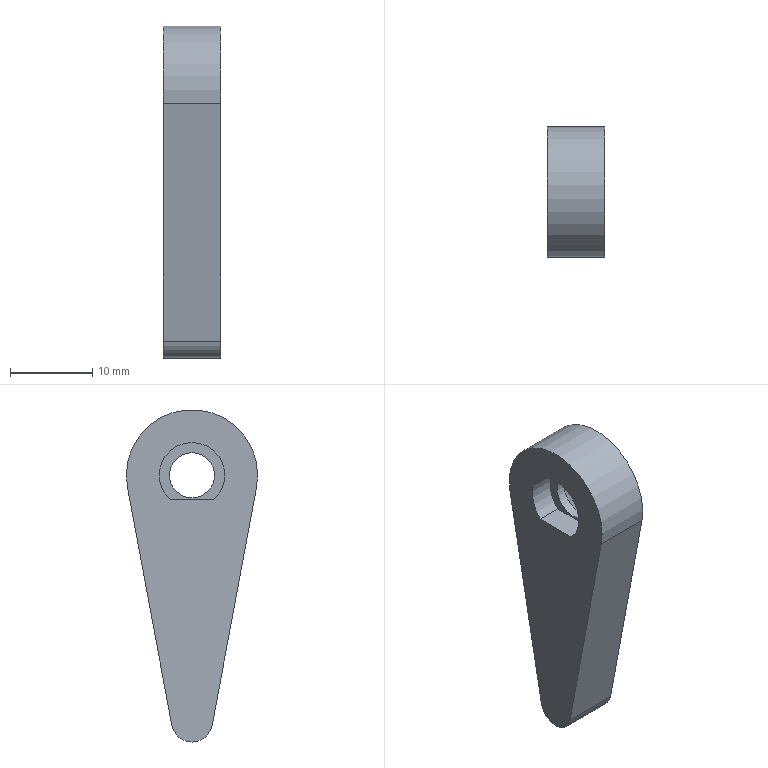Part | NX | features DATUM_CSYS 2, EXTRUDE 2, SKETCH 2, CSUNK_HOLE 1, HOLE PACKAGE 1 | 1 solid | 11 faces | box 7 x 16 x 40.5 mm | volume 2685 mm3 | plane 6 | cylinder 4 | cone 1 | commonest cylinder face diameters 5 x1 5.5 x1 8 x1 16 x1
STEP:
#1=CARTESIAN_POINT('',(0.,7.864,-1.467));
#2=VERTEX_POINT('',#1);
#3=CARTESIAN_POINT('',(0.,2.458,-30.458));
#4=VERTEX_POINT('',#3);
#5=CARTESIAN_POINT('',(0.,7.864,-1.467));
#6=DIRECTION('',(0.,-0.1833,-0.9831));
#7=VECTOR('',#6,1000.);
#8=LINE('',#5,#7);
#9=EDGE_CURVE('',#2,#4,#8,.T.);
#10=ORIENTED_EDGE('',*,*,#9,.F.);
#11=CARTESIAN_POINT('',(7.,7.864,-1.467));
#12=VERTEX_POINT('',#11);
#13=CARTESIAN_POINT('',(7.,7.864,-1.467));
#14=DIRECTION('',(-1.,0.,0.));
#15=VECTOR('',#14,1000.);
#16=LINE('',#13,#15);
#17=EDGE_CURVE('',#12,#2,#16,.T.);
#18=ORIENTED_EDGE('',*,*,#17,.F.);
#19=CARTESIAN_POINT('',(7.,2.458,-30.458));
#20=VERTEX_POINT('',#19);
#21=CARTESIAN_POINT('',(7.,7.864,-1.467));
#22=DIRECTION('',(0.,-0.1833,-0.9831));
#23=VECTOR('',#22,1000.);
#24=LINE('',#21,#23);
#25=EDGE_CURVE('',#12,#20,#24,.T.);
#26=ORIENTED_EDGE('',*,*,#25,.T.);
#27=CARTESIAN_POINT('',(7.,2.458,-30.458));
#28=DIRECTION('',(-1.,0.,0.));
#29=VECTOR('',#28,1000.);
#30=LINE('',#27,#29);
#31=EDGE_CURVE('',#20,#4,#30,.T.);
#32=ORIENTED_EDGE('',*,*,#31,.T.);
#33=EDGE_LOOP('',(#10,#18,#26,#32));
#34=FACE_BOUND('',#33,.T.);
#35=CARTESIAN_POINT('',(7.,7.864,-1.467));
#36=DIRECTION('',(0.,0.9831,-0.1833));
#37=DIRECTION('',(0.,0.1833,0.9831));
#38=AXIS2_PLACEMENT_3D('',#35,#36,#37);
#39=PLANE('',#38);
#40=ADVANCED_FACE('',(#34),#39,.T.);
#41=CARTESIAN_POINT('',(0.,-2.458,-30.458));
#42=VERTEX_POINT('',#41);
#43=CARTESIAN_POINT('',(0.,0.,-30.));
#44=DIRECTION('',(-1.,0.,0.));
#45=DIRECTION('',(0.,1.,0.));
#46=AXIS2_PLACEMENT_3D('',#43,#44,#45);
#47=CIRCLE('',#46,2.5);
#48=EDGE_CURVE('',#4,#42,#47,.T.);
#49=ORIENTED_EDGE('',*,*,#48,.F.);
#50=ORIENTED_EDGE('',*,*,#31,.F.);
#51=CARTESIAN_POINT('',(7.,-2.458,-30.458));
#52=VERTEX_POINT('',#51);
#53=CARTESIAN_POINT('',(7.,0.,-30.));
#54=DIRECTION('',(-1.,0.,0.));
#55=DIRECTION('',(0.,1.,0.));
#56=AXIS2_PLACEMENT_3D('',#53,#54,#55);
#57=CIRCLE('',#56,2.5);
#58=EDGE_CURVE('',#20,#52,#57,.T.);
#59=ORIENTED_EDGE('',*,*,#58,.T.);
#60=CARTESIAN_POINT('',(7.,-2.458,-30.458));
#61=DIRECTION('',(-1.,0.,0.));
#62=VECTOR('',#61,1000.);
#63=LINE('',#60,#62);
#64=EDGE_CURVE('',#52,#42,#63,.T.);
#65=ORIENTED_EDGE('',*,*,#64,.T.);
#66=EDGE_LOOP('',(#49,#50,#59,#65));
#67=FACE_BOUND('',#66,.T.);
#68=CARTESIAN_POINT('',(7.,0.,-30.));
#69=DIRECTION('',(-1.,0.,0.));
#70=DIRECTION('',(0.,0.,1.));
#71=AXIS2_PLACEMENT_3D('',#68,#69,#70);
#72=CYLINDRICAL_SURFACE('',#71,2.5);
#73=ADVANCED_FACE('',(#67),#72,.T.);
#74=CARTESIAN_POINT('',(0.,-7.864,-1.467));
#75=VERTEX_POINT('',#74);
#76=CARTESIAN_POINT('',(0.,-2.458,-30.458));
#77=DIRECTION('',(0.,-0.1833,0.9831));
#78=VECTOR('',#77,1000.);
#79=LINE('',#76,#78);
#80=EDGE_CURVE('',#42,#75,#79,.T.);
#81=ORIENTED_EDGE('',*,*,#80,.F.);
#82=ORIENTED_EDGE('',*,*,#64,.F.);
#83=CARTESIAN_POINT('',(7.,-7.864,-1.467));
#84=VERTEX_POINT('',#83);
#85=CARTESIAN_POINT('',(7.,-2.458,-30.458));
#86=DIRECTION('',(0.,-0.1833,0.9831));
#87=VECTOR('',#86,1000.);
#88=LINE('',#85,#87);
#89=EDGE_CURVE('',#52,#84,#88,.T.);
#90=ORIENTED_EDGE('',*,*,#89,.T.);
#91=CARTESIAN_POINT('',(7.,-7.864,-1.467));
#92=DIRECTION('',(-1.,0.,0.));
#93=VECTOR('',#92,1000.);
#94=LINE('',#91,#93);
#95=EDGE_CURVE('',#84,#75,#94,.T.);
#96=ORIENTED_EDGE('',*,*,#95,.T.);
#97=EDGE_LOOP('',(#81,#82,#90,#96));
#98=FACE_BOUND('',#97,.T.);
#99=CARTESIAN_POINT('',(7.,-2.458,-30.458));
#100=DIRECTION('',(0.,-0.9831,-0.1833));
#101=DIRECTION('',(0.,0.1833,-0.9831));
#102=AXIS2_PLACEMENT_3D('',#99,#100,#101);
#103=PLANE('',#102);
#104=ADVANCED_FACE('',(#98),#103,.T.);
#105=CARTESIAN_POINT('',(0.,0.,0.));
#106=DIRECTION('',(-1.,0.,0.));
#107=DIRECTION('',(0.,1.,0.));
#108=AXIS2_PLACEMENT_3D('',#105,#106,#107);
#109=CIRCLE('',#108,8.);
#110=EDGE_CURVE('',#75,#2,#109,.T.);
#111=ORIENTED_EDGE('',*,*,#110,.F.);
#112=ORIENTED_EDGE('',*,*,#95,.F.);
#113=CARTESIAN_POINT('',(7.,0.,0.));
#114=DIRECTION('',(-1.,0.,0.));
#115=DIRECTION('',(0.,1.,0.));
#116=AXIS2_PLACEMENT_3D('',#113,#114,#115);
#117=CIRCLE('',#116,8.);
#118=EDGE_CURVE('',#84,#12,#117,.T.);
#119=ORIENTED_EDGE('',*,*,#118,.T.);
#120=ORIENTED_EDGE('',*,*,#17,.T.);
#121=EDGE_LOOP('',(#111,#112,#119,#120));
#122=FACE_BOUND('',#121,.T.);
#123=CARTESIAN_POINT('',(7.,0.,0.));
#124=DIRECTION('',(-1.,0.,0.));
#125=DIRECTION('',(0.,0.,1.));
#126=AXIS2_PLACEMENT_3D('',#123,#124,#125);
#127=CYLINDRICAL_SURFACE('',#126,8.);
#128=ADVANCED_FACE('',(#122),#127,.T.);
#129=CARTESIAN_POINT('',(7.,0.,5.6));
#130=VERTEX_POINT('',#129);
#131=CARTESIAN_POINT('',(7.,0.,0.));
#132=DIRECTION('',(-1.,0.,0.));
#133=DIRECTION('',(0.,0.,1.));
#134=AXIS2_PLACEMENT_3D('',#131,#132,#133);
#135=CIRCLE('',#134,5.6);
#136=EDGE_CURVE('',#130,#130,#135,.T.);
#137=ORIENTED_EDGE('',*,*,#136,.T.);
#138=EDGE_LOOP('',(#137));
#139=FACE_BOUND('',#138,.T.);
#140=ORIENTED_EDGE('',*,*,#25,.F.);
#141=ORIENTED_EDGE('',*,*,#118,.F.);
#142=ORIENTED_EDGE('',*,*,#89,.F.);
#143=ORIENTED_EDGE('',*,*,#58,.F.);
#144=EDGE_LOOP('',(#140,#141,#142,#143));
#145=FACE_BOUND('',#144,.T.);
#146=CARTESIAN_POINT('',(7.,0.,-30.));
#147=DIRECTION('',(-1.,0.,0.));
#148=DIRECTION('',(0.,0.,1.));
#149=AXIS2_PLACEMENT_3D('',#146,#147,#148);
#150=PLANE('',#149);
#151=ADVANCED_FACE('',(#139,#145),#150,.F.);
#152=CARTESIAN_POINT('',(0.,2.646,-3.));
#153=VERTEX_POINT('',#152);
#154=CARTESIAN_POINT('',(0.,-2.646,-3.));
#155=VERTEX_POINT('',#154);
#156=CARTESIAN_POINT('',(0.,0.,0.));
#157=DIRECTION('',(-1.,0.,0.));
#158=DIRECTION('',(0.,1.,0.));
#159=AXIS2_PLACEMENT_3D('',#156,#157,#158);
#160=CIRCLE('',#159,4.);
#161=EDGE_CURVE('',#153,#155,#160,.F.);
#162=ORIENTED_EDGE('',*,*,#161,.T.);
#163=CARTESIAN_POINT('',(0.,2.646,-3.));
#164=DIRECTION('',(0.,-1.,0.));
#165=VECTOR('',#164,1000.);
#166=LINE('',#163,#165);
#167=EDGE_CURVE('',#155,#153,#166,.F.);
#168=ORIENTED_EDGE('',*,*,#167,.T.);
#169=EDGE_LOOP('',(#162,#168));
#170=FACE_BOUND('',#169,.T.);
#171=ORIENTED_EDGE('',*,*,#9,.T.);
#172=ORIENTED_EDGE('',*,*,#48,.T.);
#173=ORIENTED_EDGE('',*,*,#80,.T.);
#174=ORIENTED_EDGE('',*,*,#110,.T.);
#175=EDGE_LOOP('',(#171,#172,#173,#174));
#176=FACE_BOUND('',#175,.T.);
#177=CARTESIAN_POINT('',(0.,0.,-30.));
#178=DIRECTION('',(-1.,0.,0.));
#179=DIRECTION('',(0.,0.,1.));
#180=AXIS2_PLACEMENT_3D('',#177,#178,#179);
#181=PLANE('',#180);
#182=ADVANCED_FACE('',(#170,#176),#181,.T.);
#183=ORIENTED_EDGE('',*,*,#161,.F.);
#184=CARTESIAN_POINT('',(3.,2.646,-3.));
#185=VERTEX_POINT('',#184);
#186=CARTESIAN_POINT('',(3.,2.646,-3.));
#187=DIRECTION('',(-1.,0.,0.));
#188=VECTOR('',#187,1000.);
#189=LINE('',#186,#188);
#190=EDGE_CURVE('',#185,#153,#189,.T.);
#191=ORIENTED_EDGE('',*,*,#190,.F.);
#192=CARTESIAN_POINT('',(3.,-2.646,-3.));
#193=VERTEX_POINT('',#192);
#194=CARTESIAN_POINT('',(3.,0.,0.));
#195=DIRECTION('',(-1.,0.,0.));
#196=DIRECTION('',(0.,1.,0.));
#197=AXIS2_PLACEMENT_3D('',#194,#195,#196);
#198=CIRCLE('',#197,4.);
#199=EDGE_CURVE('',#193,#185,#198,.T.);
#200=ORIENTED_EDGE('',*,*,#199,.F.);
#201=CARTESIAN_POINT('',(3.,-2.646,-3.));
#202=DIRECTION('',(-1.,0.,0.));
#203=VECTOR('',#202,1000.);
#204=LINE('',#201,#203);
#205=EDGE_CURVE('',#155,#193,#204,.F.);
#206=ORIENTED_EDGE('',*,*,#205,.F.);
#207=EDGE_LOOP('',(#183,#191,#200,#206));
#208=FACE_BOUND('',#207,.T.);
#209=CARTESIAN_POINT('',(3.,0.,0.));
#210=DIRECTION('',(-1.,0.,0.));
#211=DIRECTION('',(0.,0.,1.));
#212=AXIS2_PLACEMENT_3D('',#209,#210,#211);
#213=CYLINDRICAL_SURFACE('',#212,4.);
#214=ADVANCED_FACE('',(#208),#213,.F.);
#215=ORIENTED_EDGE('',*,*,#167,.F.);
#216=ORIENTED_EDGE('',*,*,#205,.T.);
#217=CARTESIAN_POINT('',(3.,2.646,-3.));
#218=DIRECTION('',(0.,-1.,0.));
#219=VECTOR('',#218,1000.);
#220=LINE('',#217,#219);
#221=EDGE_CURVE('',#185,#193,#220,.T.);
#222=ORIENTED_EDGE('',*,*,#221,.F.);
#223=ORIENTED_EDGE('',*,*,#190,.T.);
#224=EDGE_LOOP('',(#215,#216,#222,#223));
#225=FACE_BOUND('',#224,.T.);
#226=CARTESIAN_POINT('',(3.,2.646,-3.));
#227=DIRECTION('',(0.,0.,-1.));
#228=DIRECTION('',(-1.,0.,0.));
#229=AXIS2_PLACEMENT_3D('',#226,#227,#228);
#230=PLANE('',#229);
#231=ADVANCED_FACE('',(#225),#230,.F.);
#232=CARTESIAN_POINT('',(3.,0.,2.75));
#233=VERTEX_POINT('',#232);
#234=CARTESIAN_POINT('',(3.,0.,0.));
#235=DIRECTION('',(-1.,0.,0.));
#236=DIRECTION('',(0.,0.,1.));
#237=AXIS2_PLACEMENT_3D('',#234,#235,#236);
#238=CIRCLE('',#237,2.75);
#239=EDGE_CURVE('',#233,#233,#238,.F.);
#240=ORIENTED_EDGE('',*,*,#239,.T.);
#241=EDGE_LOOP('',(#240));
#242=FACE_BOUND('',#241,.T.);
#243=ORIENTED_EDGE('',*,*,#199,.T.);
#244=ORIENTED_EDGE('',*,*,#221,.T.);
#245=EDGE_LOOP('',(#243,#244));
#246=FACE_BOUND('',#245,.T.);
#247=CARTESIAN_POINT('',(3.,0.,0.));
#248=DIRECTION('',(-1.,0.,0.));
#249=DIRECTION('',(0.,0.,1.));
#250=AXIS2_PLACEMENT_3D('',#247,#248,#249);
#251=PLANE('',#250);
#252=ADVANCED_FACE('',(#242,#246),#251,.T.);
#253=ORIENTED_EDGE('',*,*,#239,.F.);
#254=EDGE_LOOP('',(#253));
#255=FACE_BOUND('',#254,.T.);
#256=CARTESIAN_POINT('',(4.15,0.,2.75));
#257=VERTEX_POINT('',#256);
#258=CARTESIAN_POINT('',(4.15,0.,0.));
#259=DIRECTION('',(-1.,0.,0.));
#260=DIRECTION('',(0.,0.,1.));
#261=AXIS2_PLACEMENT_3D('',#258,#259,#260);
#262=CIRCLE('',#261,2.75);
#263=EDGE_CURVE('',#257,#257,#262,.F.);
#264=ORIENTED_EDGE('',*,*,#263,.T.);
#265=EDGE_LOOP('',(#264));
#266=FACE_BOUND('',#265,.T.);
#267=CARTESIAN_POINT('',(-43.,0.,0.));
#268=DIRECTION('',(-1.,0.,0.));
#269=DIRECTION('',(0.,0.,1.));
#270=AXIS2_PLACEMENT_3D('',#267,#268,#269);
#271=CYLINDRICAL_SURFACE('',#270,2.75);
#272=ADVANCED_FACE('',(#255,#266),#271,.F.);
#273=ORIENTED_EDGE('',*,*,#263,.F.);
#274=EDGE_LOOP('',(#273));
#275=FACE_BOUND('',#274,.T.);
#276=ORIENTED_EDGE('',*,*,#136,.F.);
#277=EDGE_LOOP('',(#276));
#278=FACE_BOUND('',#277,.T.);
#279=CARTESIAN_POINT('',(7.,0.,0.));
#280=DIRECTION('',(1.,0.,0.));
#281=DIRECTION('',(0.,0.,-1.));
#282=AXIS2_PLACEMENT_3D('',#279,#280,#281);
#283=CONICAL_SURFACE('',#282,5.6,0.7854);
#284=ADVANCED_FACE('',(#275,#278),#283,.F.);
#285=CLOSED_SHELL('',(#40,#73,#104,#128,#151,#182,#214,#231,#252,#272,#284));
#286=MANIFOLD_SOLID_BREP('',#285);
#287=(LENGTH_UNIT()NAMED_UNIT(*)SI_UNIT(.MILLI.,.METRE.));
#288=UNCERTAINTY_MEASURE_WITH_UNIT(LENGTH_MEASURE(0.00001),#287,'','');
#289=(NAMED_UNIT(*)PLANE_ANGLE_UNIT()SI_UNIT($,.RADIAN.));
#290=(NAMED_UNIT(*)SI_UNIT($,.STERADIAN.)SOLID_ANGLE_UNIT());
#291=(GEOMETRIC_REPRESENTATION_CONTEXT(3)GLOBAL_UNCERTAINTY_ASSIGNED_CONTEXT((#288))GLOBAL_UNIT_ASSIGNED_CONTEXT((#287,#289,#290))REPRESENTATION_CONTEXT('',''));
#292=ADVANCED_BREP_SHAPE_REPRESENTATION('',(#286),#291);